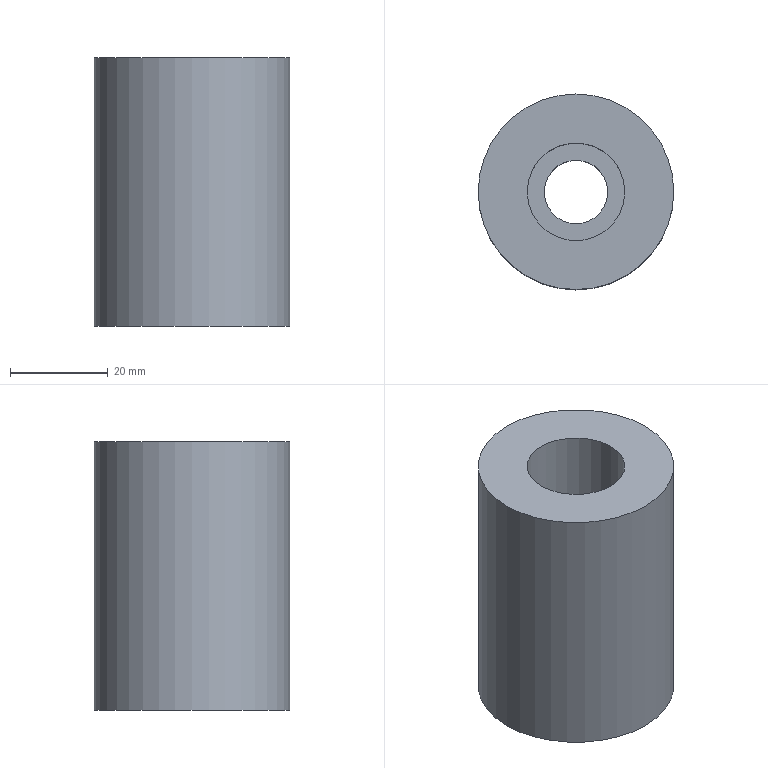Part | NX | features 模具.stp<1>[118] 2 | 1 solid | 6 faces | box 40 x 40 x 55 mm | volume 56372 mm3 | cylinder 3 | plane 3 | commonest cylinder face diameters 13 x1 20 x1 40 x1
STEP:
#1=CARTESIAN_POINT('',(10.,-220.,-135.5));
#2=VERTEX_POINT('',#1);
#3=CARTESIAN_POINT('',(0.,-220.,-135.5));
#4=DIRECTION('',(0.,0.,-1.));
#5=DIRECTION('',(1.,0.,0.));
#6=AXIS2_PLACEMENT_3D('',#3,#4,#5);
#7=CIRCLE('',#6,10.);
#8=EDGE_CURVE('',#2,#2,#7,.T.);
#9=ORIENTED_EDGE('',*,*,#8,.F.);
#10=EDGE_LOOP('',(#9));
#11=FACE_BOUND('',#10,.T.);
#12=CARTESIAN_POINT('',(10.,-220.,-165.5));
#13=VERTEX_POINT('',#12);
#14=CARTESIAN_POINT('',(0.,-220.,-165.5));
#15=DIRECTION('',(0.,0.,-1.));
#16=DIRECTION('',(1.,0.,0.));
#17=AXIS2_PLACEMENT_3D('',#14,#15,#16);
#18=CIRCLE('',#17,10.);
#19=EDGE_CURVE('',#13,#13,#18,.T.);
#20=ORIENTED_EDGE('',*,*,#19,.T.);
#21=EDGE_LOOP('',(#20));
#22=FACE_BOUND('',#21,.T.);
#23=CARTESIAN_POINT('',(0.,-220.,-135.5));
#24=DIRECTION('',(0.,0.,-1.));
#25=DIRECTION('',(1.,0.,0.));
#26=AXIS2_PLACEMENT_3D('',#23,#24,#25);
#27=CYLINDRICAL_SURFACE('',#26,10.);
#28=ADVANCED_FACE('',(#11,#22),#27,.F.);
#29=CARTESIAN_POINT('',(-6.5,-220.,-165.5));
#30=VERTEX_POINT('',#29);
#31=CARTESIAN_POINT('',(0.,-220.,-165.5));
#32=DIRECTION('',(0.,0.,1.));
#33=DIRECTION('',(-1.,0.,0.));
#34=AXIS2_PLACEMENT_3D('',#31,#32,#33);
#35=CIRCLE('',#34,6.5);
#36=EDGE_CURVE('',#30,#30,#35,.T.);
#37=ORIENTED_EDGE('',*,*,#36,.F.);
#38=EDGE_LOOP('',(#37));
#39=FACE_BOUND('',#38,.T.);
#40=ORIENTED_EDGE('',*,*,#19,.F.);
#41=EDGE_LOOP('',(#40));
#42=FACE_BOUND('',#41,.T.);
#43=CARTESIAN_POINT('',(0.,-220.,-165.5));
#44=DIRECTION('',(0.,0.,-1.));
#45=DIRECTION('',(0.,-1.,0.));
#46=AXIS2_PLACEMENT_3D('',#43,#44,#45);
#47=PLANE('',#46);
#48=ADVANCED_FACE('',(#39,#42),#47,.F.);
#49=CARTESIAN_POINT('',(6.5,-220.,-190.5));
#50=VERTEX_POINT('',#49);
#51=CARTESIAN_POINT('',(0.,-220.,-190.5));
#52=DIRECTION('',(0.,0.,1.));
#53=DIRECTION('',(1.,0.,0.));
#54=AXIS2_PLACEMENT_3D('',#51,#52,#53);
#55=CIRCLE('',#54,6.5);
#56=EDGE_CURVE('',#50,#50,#55,.T.);
#57=ORIENTED_EDGE('',*,*,#56,.F.);
#58=EDGE_LOOP('',(#57));
#59=FACE_BOUND('',#58,.T.);
#60=ORIENTED_EDGE('',*,*,#36,.T.);
#61=EDGE_LOOP('',(#60));
#62=FACE_BOUND('',#61,.T.);
#63=CARTESIAN_POINT('',(0.,-220.,-135.5));
#64=DIRECTION('',(0.,0.,-1.));
#65=DIRECTION('',(1.,0.,0.));
#66=AXIS2_PLACEMENT_3D('',#63,#64,#65);
#67=CYLINDRICAL_SURFACE('',#66,6.5);
#68=ADVANCED_FACE('',(#59,#62),#67,.F.);
#69=CARTESIAN_POINT('',(0.,-200.,-190.5));
#70=VERTEX_POINT('',#69);
#71=CARTESIAN_POINT('',(0.,-220.,-190.5));
#72=DIRECTION('',(0.,0.,1.));
#73=DIRECTION('',(0.,1.,0.));
#74=AXIS2_PLACEMENT_3D('',#71,#72,#73);
#75=CIRCLE('',#74,20.);
#76=EDGE_CURVE('',#70,#70,#75,.T.);
#77=ORIENTED_EDGE('',*,*,#76,.F.);
#78=EDGE_LOOP('',(#77));
#79=FACE_BOUND('',#78,.T.);
#80=ORIENTED_EDGE('',*,*,#56,.T.);
#81=EDGE_LOOP('',(#80));
#82=FACE_BOUND('',#81,.T.);
#83=CARTESIAN_POINT('',(0.,-220.,-190.5));
#84=DIRECTION('',(0.,0.,1.));
#85=DIRECTION('',(1.,0.,0.));
#86=AXIS2_PLACEMENT_3D('',#83,#84,#85);
#87=PLANE('',#86);
#88=ADVANCED_FACE('',(#79,#82),#87,.F.);
#89=CARTESIAN_POINT('',(20.,-220.,-135.5));
#90=VERTEX_POINT('',#89);
#91=CARTESIAN_POINT('',(0.,-220.,-135.5));
#92=DIRECTION('',(0.,0.,1.));
#93=DIRECTION('',(1.,0.,0.));
#94=AXIS2_PLACEMENT_3D('',#91,#92,#93);
#95=CIRCLE('',#94,20.);
#96=EDGE_CURVE('',#90,#90,#95,.T.);
#97=ORIENTED_EDGE('',*,*,#96,.T.);
#98=EDGE_LOOP('',(#97));
#99=FACE_BOUND('',#98,.T.);
#100=ORIENTED_EDGE('',*,*,#8,.T.);
#101=EDGE_LOOP('',(#100));
#102=FACE_BOUND('',#101,.T.);
#103=CARTESIAN_POINT('',(-250.,0.,-135.5));
#104=DIRECTION('',(0.,0.,1.));
#105=DIRECTION('',(1.,0.,0.));
#106=AXIS2_PLACEMENT_3D('',#103,#104,#105);
#107=PLANE('',#106);
#108=ADVANCED_FACE('',(#99,#102),#107,.T.);
#109=ORIENTED_EDGE('',*,*,#76,.T.);
#110=EDGE_LOOP('',(#109));
#111=FACE_BOUND('',#110,.T.);
#112=ORIENTED_EDGE('',*,*,#96,.F.);
#113=EDGE_LOOP('',(#112));
#114=FACE_BOUND('',#113,.T.);
#115=CARTESIAN_POINT('',(0.,-220.,-175.5));
#116=DIRECTION('',(0.,0.,-1.));
#117=DIRECTION('',(-1.,0.,0.));
#118=AXIS2_PLACEMENT_3D('',#115,#116,#117);
#119=CYLINDRICAL_SURFACE('',#118,20.);
#120=ADVANCED_FACE('',(#111,#114),#119,.T.);
#121=CLOSED_SHELL('',(#28,#48,#68,#88,#108,#120));
#122=MANIFOLD_SOLID_BREP('',#121);
#123=(LENGTH_UNIT()NAMED_UNIT(*)SI_UNIT(.MILLI.,.METRE.));
#124=UNCERTAINTY_MEASURE_WITH_UNIT(LENGTH_MEASURE(0.00001),#123,'','');
#125=(NAMED_UNIT(*)PLANE_ANGLE_UNIT()SI_UNIT($,.RADIAN.));
#126=(NAMED_UNIT(*)SI_UNIT($,.STERADIAN.)SOLID_ANGLE_UNIT());
#127=(GEOMETRIC_REPRESENTATION_CONTEXT(3)GLOBAL_UNCERTAINTY_ASSIGNED_CONTEXT((#124))GLOBAL_UNIT_ASSIGNED_CONTEXT((#123,#125,#126))REPRESENTATION_CONTEXT('',''));
#128=ADVANCED_BREP_SHAPE_REPRESENTATION('',(#122),#127);